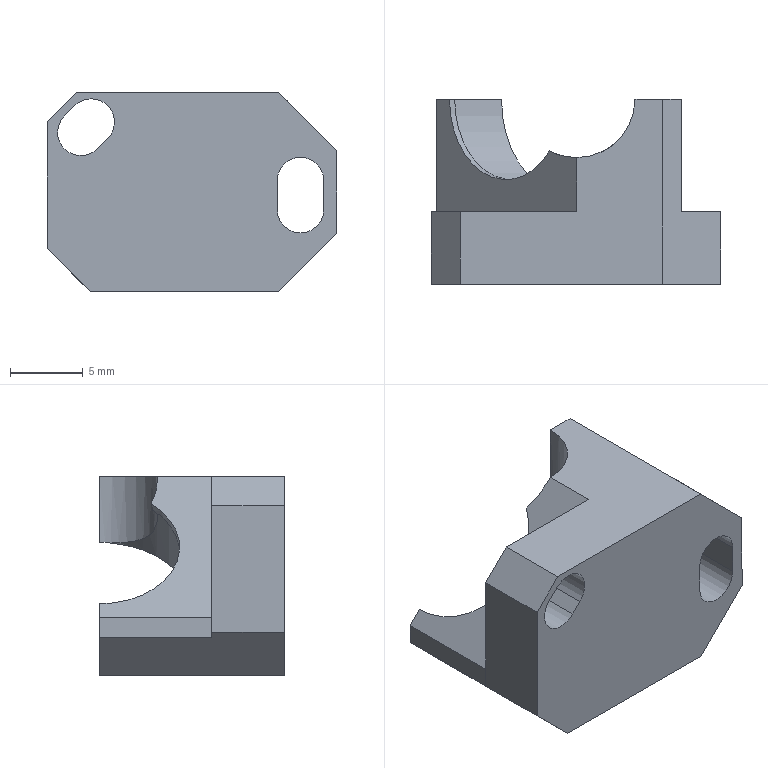Part | SolidWorks | features ICE 10, Chamfer 3, Extrusion 1, MoveFace 1 | 1 solid | 30 faces | box 19.9 x 12.7 x 13.659 mm | volume 1490 mm3 | plane 21 | cylinder 9 | commonest cylinder face diameters 3.2 x6 8 x1 11 x1 12.9 x1
STEP:
#1=CARTESIAN_POINT('',(8.727,0.,19.173));
#2=VERTEX_POINT('',#1);
#3=CARTESIAN_POINT('',(9.858,0.,16.442));
#4=VERTEX_POINT('',#3);
#5=CARTESIAN_POINT('',(8.727,0.,17.573));
#6=DIRECTION('',(0.,1.,0.));
#7=DIRECTION('',(0.,0.,1.));
#8=AXIS2_PLACEMENT_3D('',#5,#6,#7);
#9=CIRCLE('',#8,1.6);
#10=EDGE_CURVE('',#2,#4,#9,.T.);
#11=ORIENTED_EDGE('',*,*,#10,.F.);
#12=CARTESIAN_POINT('',(8.727,5.,19.173));
#13=VERTEX_POINT('',#12);
#14=CARTESIAN_POINT('',(8.727,-5.,19.173));
#15=DIRECTION('',(0.,1.,0.));
#16=VECTOR('',#15,1000.);
#17=LINE('',#14,#16);
#18=EDGE_CURVE('',#2,#13,#17,.T.);
#19=ORIENTED_EDGE('',*,*,#18,.T.);
#20=CARTESIAN_POINT('',(9.858,5.,16.442));
#21=VERTEX_POINT('',#20);
#22=CARTESIAN_POINT('',(8.727,5.,17.573));
#23=DIRECTION('',(0.,1.,0.));
#24=DIRECTION('',(0.,0.,1.));
#25=AXIS2_PLACEMENT_3D('',#22,#23,#24);
#26=CIRCLE('',#25,1.6);
#27=EDGE_CURVE('',#13,#21,#26,.T.);
#28=ORIENTED_EDGE('',*,*,#27,.T.);
#29=CARTESIAN_POINT('',(9.858,-5.,16.442));
#30=DIRECTION('',(0.,1.,0.));
#31=VECTOR('',#30,1000.);
#32=LINE('',#29,#31);
#33=EDGE_CURVE('',#4,#21,#32,.T.);
#34=ORIENTED_EDGE('',*,*,#33,.F.);
#35=EDGE_LOOP('',(#11,#19,#28,#34));
#36=FACE_OUTER_BOUND('',#35,.T.);
#37=CARTESIAN_POINT('',(8.727,-5.,17.573));
#38=DIRECTION('',(0.,1.,0.));
#39=DIRECTION('',(0.,0.,1.));
#40=AXIS2_PLACEMENT_3D('',#37,#38,#39);
#41=CYLINDRICAL_SURFACE('',#40,1.6);
#42=ADVANCED_FACE('',(#36),#41,.F.);
#43=CARTESIAN_POINT('',(23.1,0.,15.154));
#44=VERTEX_POINT('',#43);
#45=CARTESIAN_POINT('',(24.7,0.,13.554));
#46=VERTEX_POINT('',#45);
#47=CARTESIAN_POINT('',(23.1,0.,13.554));
#48=DIRECTION('',(0.,1.,0.));
#49=DIRECTION('',(0.,0.,1.));
#50=AXIS2_PLACEMENT_3D('',#47,#48,#49);
#51=CIRCLE('',#50,1.6);
#52=EDGE_CURVE('',#44,#46,#51,.T.);
#53=ORIENTED_EDGE('',*,*,#52,.F.);
#54=CARTESIAN_POINT('',(23.1,5.,15.154));
#55=VERTEX_POINT('',#54);
#56=CARTESIAN_POINT('',(23.1,-0.5,15.154));
#57=DIRECTION('',(0.,1.,0.));
#58=VECTOR('',#57,1000.);
#59=LINE('',#56,#58);
#60=EDGE_CURVE('',#44,#55,#59,.T.);
#61=ORIENTED_EDGE('',*,*,#60,.T.);
#62=CARTESIAN_POINT('',(24.7,5.,13.554));
#63=VERTEX_POINT('',#62);
#64=CARTESIAN_POINT('',(23.1,5.,13.554));
#65=DIRECTION('',(0.,1.,0.));
#66=DIRECTION('',(0.,0.,1.));
#67=AXIS2_PLACEMENT_3D('',#64,#65,#66);
#68=CIRCLE('',#67,1.6);
#69=EDGE_CURVE('',#55,#63,#68,.T.);
#70=ORIENTED_EDGE('',*,*,#69,.T.);
#71=CARTESIAN_POINT('',(24.7,-0.5,13.554));
#72=DIRECTION('',(0.,1.,0.));
#73=VECTOR('',#72,1000.);
#74=LINE('',#71,#73);
#75=EDGE_CURVE('',#46,#63,#74,.T.);
#76=ORIENTED_EDGE('',*,*,#75,.F.);
#77=EDGE_LOOP('',(#53,#61,#70,#76));
#78=FACE_OUTER_BOUND('',#77,.T.);
#79=CARTESIAN_POINT('',(23.1,-0.5,13.554));
#80=DIRECTION('',(0.,1.,0.));
#81=DIRECTION('',(0.,0.,1.));
#82=AXIS2_PLACEMENT_3D('',#79,#80,#81);
#83=CYLINDRICAL_SURFACE('',#82,1.6);
#84=ADVANCED_FACE('',(#78),#83,.F.);
#85=CARTESIAN_POINT('',(13.83,9.163,17.727));
#86=VERTEX_POINT('',#85);
#87=CARTESIAN_POINT('',(6.963,12.7,10.859));
#88=VERTEX_POINT('',#87);
#89=CARTESIAN_POINT('',(10.852,12.7,14.748));
#90=DIRECTION('',(0.7071,0.,-0.7071));
#91=DIRECTION('',(-0.7071,0.,-0.7071));
#92=AXIS2_PLACEMENT_3D('',#89,#90,#91);
#93=CIRCLE('',#92,5.5);
#94=EDGE_CURVE('',#86,#88,#93,.T.);
#95=ORIENTED_EDGE('',*,*,#94,.F.);
#96=CARTESIAN_POINT('',(14.106,9.031,17.288));
#97=VERTEX_POINT('',#96);
#98=CARTESIAN_POINT('',(13.83,9.163,17.727));
#99=CARTESIAN_POINT('',(13.92,9.116,17.58));
#100=CARTESIAN_POINT('',(14.012,9.072,17.434));
#101=CARTESIAN_POINT('',(14.106,9.031,17.288));
#102=B_SPLINE_CURVE_WITH_KNOTS('',3,(#98,#99,#100,#101),.UNSPECIFIED.,.F.,.F.,(4,4),(0.0005321,0.001067),.UNSPECIFIED.);
#103=EDGE_CURVE('',#86,#97,#102,.T.);
#104=ORIENTED_EDGE('',*,*,#103,.T.);
#105=CARTESIAN_POINT('',(7.32,12.7,10.502));
#106=VERTEX_POINT('',#105);
#107=CARTESIAN_POINT('',(11.209,12.7,14.391));
#108=DIRECTION('',(-0.7071,0.,0.7071));
#109=DIRECTION('',(-0.7071,0.,-0.7071));
#110=AXIS2_PLACEMENT_3D('',#107,#108,#109);
#111=CIRCLE('',#110,5.5);
#112=EDGE_CURVE('',#106,#97,#111,.T.);
#113=ORIENTED_EDGE('',*,*,#112,.F.);
#114=CARTESIAN_POINT('',(5.764,12.7,12.058));
#115=DIRECTION('',(-0.7071,0.,0.7071));
#116=VECTOR('',#115,1000.);
#117=LINE('',#114,#116);
#118=EDGE_CURVE('',#106,#88,#117,.T.);
#119=ORIENTED_EDGE('',*,*,#118,.T.);
#120=EDGE_LOOP('',(#95,#104,#113,#119));
#121=FACE_OUTER_BOUND('',#120,.T.);
#122=CARTESIAN_POINT('',(9.653,12.7,15.947));
#123=DIRECTION('',(0.7071,0.,-0.7071));
#124=DIRECTION('',(-0.7071,0.,-0.7071));
#125=AXIS2_PLACEMENT_3D('',#122,#123,#124);
#126=CYLINDRICAL_SURFACE('',#125,5.5);
#127=ADVANCED_FACE('',(#121),#126,.F.);
#128=CARTESIAN_POINT('',(19.699,12.7,19.6));
#129=VERTEX_POINT('',#128);
#130=CARTESIAN_POINT('',(19.699,12.7,15.103));
#131=VERTEX_POINT('',#130);
#132=CARTESIAN_POINT('',(19.699,12.7,5.6));
#133=DIRECTION('',(0.,0.,-1.));
#134=VECTOR('',#133,1000.);
#135=LINE('',#132,#134);
#136=EDGE_CURVE('',#129,#131,#135,.T.);
#137=ORIENTED_EDGE('',*,*,#136,.F.);
#138=CARTESIAN_POINT('',(21.6,12.7,19.6));
#139=VERTEX_POINT('',#138);
#140=CARTESIAN_POINT('',(0.,12.7,19.6));
#141=DIRECTION('',(-1.,0.,0.));
#142=VECTOR('',#141,1000.);
#143=LINE('',#140,#142);
#144=EDGE_CURVE('',#139,#129,#143,.T.);
#145=ORIENTED_EDGE('',*,*,#144,.F.);
#146=CARTESIAN_POINT('',(22.898,12.7,18.302));
#147=VERTEX_POINT('',#146);
#148=CARTESIAN_POINT('',(21.6,12.7,19.6));
#149=DIRECTION('',(-0.7071,0.,0.7071));
#150=VECTOR('',#149,1000.);
#151=LINE('',#148,#150);
#152=EDGE_CURVE('',#147,#139,#151,.T.);
#153=ORIENTED_EDGE('',*,*,#152,.F.);
#154=CARTESIAN_POINT('',(25.6,12.7,21.004));
#155=DIRECTION('',(-0.7071,0.,-0.7071));
#156=VECTOR('',#155,1000.);
#157=LINE('',#154,#156);
#158=EDGE_CURVE('',#147,#131,#157,.T.);
#159=ORIENTED_EDGE('',*,*,#158,.T.);
#160=EDGE_LOOP('',(#137,#145,#153,#159));
#161=FACE_OUTER_BOUND('',#160,.T.);
#162=CARTESIAN_POINT('',(0.,12.7,0.));
#163=DIRECTION('',(0.,1.,0.));
#164=DIRECTION('',(0.,0.,1.));
#165=AXIS2_PLACEMENT_3D('',#162,#163,#164);
#166=PLANE('',#165);
#167=ADVANCED_FACE('',(#161),#166,.T.);
#168=CARTESIAN_POINT('',(25.6,5.,15.6));
#169=VERTEX_POINT('',#168);
#170=CARTESIAN_POINT('',(22.898,5.,18.302));
#171=VERTEX_POINT('',#170);
#172=CARTESIAN_POINT('',(20.6,5.,20.6));
#173=DIRECTION('',(-0.7071,0.,0.7071));
#174=VECTOR('',#173,1000.);
#175=LINE('',#172,#174);
#176=EDGE_CURVE('',#169,#171,#175,.T.);
#177=ORIENTED_EDGE('',*,*,#176,.F.);
#178=CARTESIAN_POINT('',(25.6,5.,9.941));
#179=VERTEX_POINT('',#178);
#180=CARTESIAN_POINT('',(25.6,5.,0.));
#181=DIRECTION('',(0.,0.,-1.));
#182=VECTOR('',#181,1000.);
#183=LINE('',#180,#182);
#184=EDGE_CURVE('',#169,#179,#183,.T.);
#185=ORIENTED_EDGE('',*,*,#184,.T.);
#186=CARTESIAN_POINT('',(21.6,5.,5.941));
#187=VERTEX_POINT('',#186);
#188=CARTESIAN_POINT('',(7.829,5.,-7.829));
#189=DIRECTION('',(-0.7071,0.,-0.7071));
#190=VECTOR('',#189,1000.);
#191=LINE('',#188,#190);
#192=EDGE_CURVE('',#179,#187,#191,.T.);
#193=ORIENTED_EDGE('',*,*,#192,.T.);
#194=CARTESIAN_POINT('',(10.537,5.,5.941));
#195=VERTEX_POINT('',#194);
#196=CARTESIAN_POINT('',(0.,5.,5.941));
#197=DIRECTION('',(1.,0.,0.));
#198=VECTOR('',#197,1000.);
#199=LINE('',#196,#198);
#200=EDGE_CURVE('',#195,#187,#199,.T.);
#201=ORIENTED_EDGE('',*,*,#200,.F.);
#202=CARTESIAN_POINT('',(15.098,5.,10.502));
#203=DIRECTION('',(-0.7071,0.,-0.7071));
#204=VECTOR('',#203,1000.);
#205=LINE('',#202,#204);
#206=EDGE_CURVE('',#171,#195,#205,.T.);
#207=ORIENTED_EDGE('',*,*,#206,.F.);
#208=EDGE_LOOP('',(#177,#185,#193,#201,#207));
#209=FACE_OUTER_BOUND('',#208,.T.);
#210=CARTESIAN_POINT('',(21.5,5.,13.554));
#211=VERTEX_POINT('',#210);
#212=CARTESIAN_POINT('',(23.1,5.,13.554));
#213=DIRECTION('',(0.,1.,0.));
#214=DIRECTION('',(0.,0.,1.));
#215=AXIS2_PLACEMENT_3D('',#212,#213,#214);
#216=CIRCLE('',#215,1.6);
#217=EDGE_CURVE('',#211,#55,#216,.T.);
#218=ORIENTED_EDGE('',*,*,#217,.F.);
#219=CARTESIAN_POINT('',(21.5,5.,11.554));
#220=VERTEX_POINT('',#219);
#221=CARTESIAN_POINT('',(21.5,5.,13.554));
#222=DIRECTION('',(0.,0.,1.));
#223=VECTOR('',#222,1000.);
#224=LINE('',#221,#223);
#225=EDGE_CURVE('',#220,#211,#224,.T.);
#226=ORIENTED_EDGE('',*,*,#225,.F.);
#227=CARTESIAN_POINT('',(24.7,5.,11.554));
#228=VERTEX_POINT('',#227);
#229=CARTESIAN_POINT('',(23.1,5.,11.554));
#230=DIRECTION('',(0.,1.,0.));
#231=DIRECTION('',(0.,0.,1.));
#232=AXIS2_PLACEMENT_3D('',#229,#230,#231);
#233=CIRCLE('',#232,1.6);
#234=EDGE_CURVE('',#228,#220,#233,.T.);
#235=ORIENTED_EDGE('',*,*,#234,.F.);
#236=CARTESIAN_POINT('',(24.7,5.,13.554));
#237=DIRECTION('',(0.,0.,-1.));
#238=VECTOR('',#237,1000.);
#239=LINE('',#236,#238);
#240=EDGE_CURVE('',#63,#228,#239,.T.);
#241=ORIENTED_EDGE('',*,*,#240,.F.);
#242=ORIENTED_EDGE('',*,*,#69,.F.);
#243=EDGE_LOOP('',(#218,#226,#235,#241,#242));
#244=FACE_BOUND('',#243,.T.);
#245=CARTESIAN_POINT('',(0.,5.,0.));
#246=DIRECTION('',(0.,1.,0.));
#247=DIRECTION('',(0.,0.,1.));
#248=AXIS2_PLACEMENT_3D('',#245,#246,#247);
#249=PLANE('',#248);
#250=ADVANCED_FACE('',(#209,#244),#249,.T.);
#251=CARTESIAN_POINT('',(5.7,5.,17.6));
#252=VERTEX_POINT('',#251);
#253=CARTESIAN_POINT('',(5.7,5.,8.896));
#254=VERTEX_POINT('',#253);
#255=CARTESIAN_POINT('',(5.7,5.,0.));
#256=DIRECTION('',(0.,0.,-1.));
#257=VECTOR('',#256,1000.);
#258=LINE('',#255,#257);
#259=EDGE_CURVE('',#252,#254,#258,.T.);
#260=ORIENTED_EDGE('',*,*,#259,.F.);
#261=CARTESIAN_POINT('',(7.7,5.,19.6));
#262=VERTEX_POINT('',#261);
#263=CARTESIAN_POINT('',(-5.6,5.,6.3));
#264=DIRECTION('',(0.7071,0.,0.7071));
#265=VECTOR('',#264,1000.);
#266=LINE('',#263,#265);
#267=EDGE_CURVE('',#252,#262,#266,.T.);
#268=ORIENTED_EDGE('',*,*,#267,.T.);
#269=CARTESIAN_POINT('',(15.704,5.,19.6));
#270=VERTEX_POINT('',#269);
#271=CARTESIAN_POINT('',(0.,5.,19.6));
#272=DIRECTION('',(-1.,0.,0.));
#273=VECTOR('',#272,1000.);
#274=LINE('',#271,#273);
#275=EDGE_CURVE('',#270,#262,#274,.T.);
#276=ORIENTED_EDGE('',*,*,#275,.F.);
#277=CARTESIAN_POINT('',(6.054,5.,9.95));
#278=VERTEX_POINT('',#277);
#279=CARTESIAN_POINT('',(0.7,5.,4.596));
#280=DIRECTION('',(0.7071,0.,0.7071));
#281=VECTOR('',#280,1000.);
#282=LINE('',#279,#281);
#283=EDGE_CURVE('',#278,#270,#282,.T.);
#284=ORIENTED_EDGE('',*,*,#283,.F.);
#285=CARTESIAN_POINT('',(6.054,5.,8.543));
#286=VERTEX_POINT('',#285);
#287=CARTESIAN_POINT('',(6.054,5.,9.95));
#288=DIRECTION('',(0.,0.,-1.));
#289=VECTOR('',#288,1000.);
#290=LINE('',#287,#289);
#291=EDGE_CURVE('',#278,#286,#290,.T.);
#292=ORIENTED_EDGE('',*,*,#291,.T.);
#293=CARTESIAN_POINT('',(7.298,5.,7.298));
#294=DIRECTION('',(0.7071,0.,-0.7071));
#295=VECTOR('',#294,1000.);
#296=LINE('',#293,#295);
#297=EDGE_CURVE('',#254,#286,#296,.T.);
#298=ORIENTED_EDGE('',*,*,#297,.F.);
#299=EDGE_LOOP('',(#260,#268,#276,#284,#292,#298));
#300=FACE_OUTER_BOUND('',#299,.T.);
#301=CARTESIAN_POINT('',(7.596,5.,18.704));
#302=VERTEX_POINT('',#301);
#303=CARTESIAN_POINT('',(8.727,5.,17.573));
#304=DIRECTION('',(0.,1.,0.));
#305=DIRECTION('',(0.,0.,1.));
#306=AXIS2_PLACEMENT_3D('',#303,#304,#305);
#307=CIRCLE('',#306,1.6);
#308=EDGE_CURVE('',#302,#13,#307,.T.);
#309=ORIENTED_EDGE('',*,*,#308,.F.);
#310=CARTESIAN_POINT('',(6.889,5.,17.997));
#311=VERTEX_POINT('',#310);
#312=CARTESIAN_POINT('',(6.889,5.,17.997));
#313=DIRECTION('',(0.7071,0.,0.7071));
#314=VECTOR('',#313,1000.);
#315=LINE('',#312,#314);
#316=EDGE_CURVE('',#311,#302,#315,.T.);
#317=ORIENTED_EDGE('',*,*,#316,.F.);
#318=CARTESIAN_POINT('',(9.151,5.,15.734));
#319=VERTEX_POINT('',#318);
#320=CARTESIAN_POINT('',(8.02,5.,16.866));
#321=DIRECTION('',(0.,1.,0.));
#322=DIRECTION('',(0.,0.,1.));
#323=AXIS2_PLACEMENT_3D('',#320,#321,#322);
#324=CIRCLE('',#323,1.6);
#325=EDGE_CURVE('',#319,#311,#324,.T.);
#326=ORIENTED_EDGE('',*,*,#325,.F.);
#327=CARTESIAN_POINT('',(9.858,5.,16.442));
#328=DIRECTION('',(-0.7071,0.,-0.7071));
#329=VECTOR('',#328,1000.);
#330=LINE('',#327,#329);
#331=EDGE_CURVE('',#21,#319,#330,.T.);
#332=ORIENTED_EDGE('',*,*,#331,.F.);
#333=ORIENTED_EDGE('',*,*,#27,.F.);
#334=EDGE_LOOP('',(#309,#317,#326,#332,#333));
#335=FACE_BOUND('',#334,.T.);
#336=CARTESIAN_POINT('',(0.,5.,0.));
#337=DIRECTION('',(0.,1.,0.));
#338=DIRECTION('',(0.,0.,1.));
#339=AXIS2_PLACEMENT_3D('',#336,#337,#338);
#340=PLANE('',#339);
#341=ADVANCED_FACE('',(#300,#335),#340,.T.);
#342=ORIENTED_EDGE('',*,*,#184,.F.);
#343=CARTESIAN_POINT('',(25.6,0.,15.6));
#344=VERTEX_POINT('',#343);
#345=CARTESIAN_POINT('',(25.6,-17.8,15.6));
#346=DIRECTION('',(0.,1.,0.));
#347=VECTOR('',#346,1000.);
#348=LINE('',#345,#347);
#349=EDGE_CURVE('',#344,#169,#348,.T.);
#350=ORIENTED_EDGE('',*,*,#349,.F.);
#351=CARTESIAN_POINT('',(25.6,0.,9.941));
#352=VERTEX_POINT('',#351);
#353=CARTESIAN_POINT('',(25.6,0.,0.));
#354=DIRECTION('',(0.,0.,-1.));
#355=VECTOR('',#354,1000.);
#356=LINE('',#353,#355);
#357=EDGE_CURVE('',#344,#352,#356,.T.);
#358=ORIENTED_EDGE('',*,*,#357,.T.);
#359=CARTESIAN_POINT('',(25.6,5.,9.941));
#360=DIRECTION('',(0.,1.,0.));
#361=VECTOR('',#360,1000.);
#362=LINE('',#359,#361);
#363=EDGE_CURVE('',#352,#179,#362,.T.);
#364=ORIENTED_EDGE('',*,*,#363,.T.);
#365=EDGE_LOOP('',(#342,#350,#358,#364));
#366=FACE_OUTER_BOUND('',#365,.T.);
#367=CARTESIAN_POINT('',(25.6,5.,0.));
#368=DIRECTION('',(-1.,0.,0.));
#369=DIRECTION('',(0.,0.,1.));
#370=AXIS2_PLACEMENT_3D('',#367,#368,#369);
#371=PLANE('',#370);
#372=ADVANCED_FACE('',(#366),#371,.F.);
#373=CARTESIAN_POINT('',(6.889,0.,17.997));
#374=VERTEX_POINT('',#373);
#375=CARTESIAN_POINT('',(7.596,0.,18.704));
#376=VERTEX_POINT('',#375);
#377=CARTESIAN_POINT('',(-5.204,0.,5.904));
#378=DIRECTION('',(0.7071,0.,0.7071));
#379=VECTOR('',#378,1000.);
#380=LINE('',#377,#379);
#381=EDGE_CURVE('',#374,#376,#380,.T.);
#382=ORIENTED_EDGE('',*,*,#381,.T.);
#383=CARTESIAN_POINT('',(8.727,0.,17.573));
#384=DIRECTION('',(0.,1.,0.));
#385=DIRECTION('',(0.,0.,1.));
#386=AXIS2_PLACEMENT_3D('',#383,#384,#385);
#387=CIRCLE('',#386,1.6);
#388=EDGE_CURVE('',#376,#2,#387,.T.);
#389=ORIENTED_EDGE('',*,*,#388,.T.);
#390=ORIENTED_EDGE('',*,*,#10,.T.);
#391=CARTESIAN_POINT('',(9.151,0.,15.734));
#392=VERTEX_POINT('',#391);
#393=CARTESIAN_POINT('',(-2.942,0.,3.642));
#394=DIRECTION('',(-0.7071,0.,-0.7071));
#395=VECTOR('',#394,1000.);
#396=LINE('',#393,#395);
#397=EDGE_CURVE('',#4,#392,#396,.T.);
#398=ORIENTED_EDGE('',*,*,#397,.T.);
#399=CARTESIAN_POINT('',(8.02,0.,16.866));
#400=DIRECTION('',(0.,1.,0.));
#401=DIRECTION('',(0.,0.,1.));
#402=AXIS2_PLACEMENT_3D('',#399,#400,#401);
#403=CIRCLE('',#402,1.6);
#404=EDGE_CURVE('',#392,#374,#403,.T.);
#405=ORIENTED_EDGE('',*,*,#404,.T.);
#406=EDGE_LOOP('',(#382,#389,#390,#398,#405));
#407=FACE_BOUND('',#406,.T.);
#408=CARTESIAN_POINT('',(21.5,0.,11.554));
#409=VERTEX_POINT('',#408);
#410=CARTESIAN_POINT('',(21.5,0.,13.554));
#411=VERTEX_POINT('',#410);
#412=CARTESIAN_POINT('',(21.5,0.,0.));
#413=DIRECTION('',(0.,0.,1.));
#414=VECTOR('',#413,1000.);
#415=LINE('',#412,#414);
#416=EDGE_CURVE('',#409,#411,#415,.T.);
#417=ORIENTED_EDGE('',*,*,#416,.T.);
#418=CARTESIAN_POINT('',(23.1,0.,13.554));
#419=DIRECTION('',(0.,1.,0.));
#420=DIRECTION('',(0.,0.,1.));
#421=AXIS2_PLACEMENT_3D('',#418,#419,#420);
#422=CIRCLE('',#421,1.6);
#423=EDGE_CURVE('',#411,#44,#422,.T.);
#424=ORIENTED_EDGE('',*,*,#423,.T.);
#425=ORIENTED_EDGE('',*,*,#52,.T.);
#426=CARTESIAN_POINT('',(24.7,0.,11.554));
#427=VERTEX_POINT('',#426);
#428=CARTESIAN_POINT('',(24.7,0.,0.));
#429=DIRECTION('',(0.,0.,-1.));
#430=VECTOR('',#429,1000.);
#431=LINE('',#428,#430);
#432=EDGE_CURVE('',#46,#427,#431,.T.);
#433=ORIENTED_EDGE('',*,*,#432,.T.);
#434=CARTESIAN_POINT('',(23.1,0.,11.554));
#435=DIRECTION('',(0.,1.,0.));
#436=DIRECTION('',(0.,0.,1.));
#437=AXIS2_PLACEMENT_3D('',#434,#435,#436);
#438=CIRCLE('',#437,1.6);
#439=EDGE_CURVE('',#427,#409,#438,.T.);
#440=ORIENTED_EDGE('',*,*,#439,.T.);
#441=EDGE_LOOP('',(#417,#424,#425,#433,#440));
#442=FACE_BOUND('',#441,.T.);
#443=CARTESIAN_POINT('',(21.6,0.,19.6));
#444=VERTEX_POINT('',#443);
#445=CARTESIAN_POINT('',(7.7,0.,19.6));
#446=VERTEX_POINT('',#445);
#447=CARTESIAN_POINT('',(0.,0.,19.6));
#448=DIRECTION('',(-1.,0.,0.));
#449=VECTOR('',#448,1000.);
#450=LINE('',#447,#449);
#451=EDGE_CURVE('',#444,#446,#450,.T.);
#452=ORIENTED_EDGE('',*,*,#451,.T.);
#453=CARTESIAN_POINT('',(5.7,0.,17.6));
#454=VERTEX_POINT('',#453);
#455=CARTESIAN_POINT('',(7.7,0.,19.6));
#456=DIRECTION('',(-0.7071,0.,-0.7071));
#457=VECTOR('',#456,1000.);
#458=LINE('',#455,#457);
#459=EDGE_CURVE('',#446,#454,#458,.T.);
#460=ORIENTED_EDGE('',*,*,#459,.T.);
#461=CARTESIAN_POINT('',(5.7,0.,8.896));
#462=VERTEX_POINT('',#461);
#463=CARTESIAN_POINT('',(5.7,0.,0.));
#464=DIRECTION('',(0.,0.,-1.));
#465=VECTOR('',#464,1000.);
#466=LINE('',#463,#465);
#467=EDGE_CURVE('',#454,#462,#466,.T.);
#468=ORIENTED_EDGE('',*,*,#467,.T.);
#469=CARTESIAN_POINT('',(8.655,0.,5.941));
#470=VERTEX_POINT('',#469);
#471=CARTESIAN_POINT('',(7.298,0.,7.298));
#472=DIRECTION('',(0.7071,0.,-0.7071));
#473=VECTOR('',#472,1000.);
#474=LINE('',#471,#473);
#475=EDGE_CURVE('',#462,#470,#474,.T.);
#476=ORIENTED_EDGE('',*,*,#475,.T.);
#477=CARTESIAN_POINT('',(21.6,0.,5.941));
#478=VERTEX_POINT('',#477);
#479=CARTESIAN_POINT('',(0.,0.,5.941));
#480=DIRECTION('',(1.,0.,0.));
#481=VECTOR('',#480,1000.);
#482=LINE('',#479,#481);
#483=EDGE_CURVE('',#470,#478,#482,.T.);
#484=ORIENTED_EDGE('',*,*,#483,.T.);
#485=CARTESIAN_POINT('',(25.6,0.,9.941));
#486=DIRECTION('',(0.7071,0.,0.7071));
#487=VECTOR('',#486,1000.);
#488=LINE('',#485,#487);
#489=EDGE_CURVE('',#478,#352,#488,.T.);
#490=ORIENTED_EDGE('',*,*,#489,.T.);
#491=ORIENTED_EDGE('',*,*,#357,.F.);
#492=CARTESIAN_POINT('',(20.6,0.,20.6));
#493=DIRECTION('',(-0.7071,0.,0.7071));
#494=VECTOR('',#493,1000.);
#495=LINE('',#492,#494);
#496=EDGE_CURVE('',#344,#444,#495,.T.);
#497=ORIENTED_EDGE('',*,*,#496,.T.);
#498=EDGE_LOOP('',(#452,#460,#468,#476,#484,#490,#491,#497));
#499=FACE_OUTER_BOUND('',#498,.T.);
#500=CARTESIAN_POINT('',(0.,0.,0.));
#501=DIRECTION('',(0.,1.,0.));
#502=DIRECTION('',(0.,0.,1.));
#503=AXIS2_PLACEMENT_3D('',#500,#501,#502);
#504=PLANE('',#503);
#505=ADVANCED_FACE('',(#407,#442,#499),#504,.F.);
#506=CARTESIAN_POINT('',(19.628,11.948,15.032));
#507=VERTEX_POINT('',#506);
#508=CARTESIAN_POINT('',(10.537,12.7,5.941));
#509=VERTEX_POINT('',#508);
#510=CARTESIAN_POINT('',(15.098,12.7,10.502));
#511=DIRECTION('',(0.7071,0.,-0.7071));
#512=DIRECTION('',(-0.7071,0.,-0.7071));
#513=AXIS2_PLACEMENT_3D('',#510,#511,#512);
#514=CIRCLE('',#513,6.45);
#515=EDGE_CURVE('',#507,#509,#514,.T.);
#516=ORIENTED_EDGE('',*,*,#515,.F.);
#517=CARTESIAN_POINT('',(19.628,11.948,15.032));
#518=CARTESIAN_POINT('',(19.675,12.196,15.079));
#519=CARTESIAN_POINT('',(19.699,12.448,15.103));
#520=CARTESIAN_POINT('',(19.699,12.7,15.103));
#521=(BOUNDED_CURVE()B_SPLINE_CURVE(3,(#517,#518,#519,#520),.UNSPECIFIED.,.F.,.F.)B_SPLINE_CURVE_WITH_KNOTS((4,4),(6.094,6.283),.UNSPECIFIED.)CURVE()GEOMETRIC_REPRESENTATION_ITEM()RATIONAL_B_SPLINE_CURVE((1.,0.997,0.997,1.))REPRESENTATION_ITEM(''));
#522=EDGE_CURVE('',#507,#131,#521,.T.);
#523=ORIENTED_EDGE('',*,*,#522,.T.);
#524=ORIENTED_EDGE('',*,*,#158,.F.);
#525=CARTESIAN_POINT('',(22.898,12.7,18.302));
#526=DIRECTION('',(0.,-1.,0.));
#527=VECTOR('',#526,1000.);
#528=LINE('',#525,#527);
#529=EDGE_CURVE('',#147,#171,#528,.T.);
#530=ORIENTED_EDGE('',*,*,#529,.T.);
#531=ORIENTED_EDGE('',*,*,#206,.T.);
#532=CARTESIAN_POINT('',(10.537,12.7,5.941));
#533=DIRECTION('',(0.,1.,0.));
#534=VECTOR('',#533,1000.);
#535=LINE('',#532,#534);
#536=EDGE_CURVE('',#195,#509,#535,.T.);
#537=ORIENTED_EDGE('',*,*,#536,.T.);
#538=EDGE_LOOP('',(#516,#523,#524,#530,#531,#537));
#539=FACE_OUTER_BOUND('',#538,.T.);
#540=CARTESIAN_POINT('',(15.098,12.7,10.502));
#541=DIRECTION('',(-0.7071,0.,0.7071));
#542=DIRECTION('',(0.7071,0.,0.7071));
#543=AXIS2_PLACEMENT_3D('',#540,#541,#542);
#544=PLANE('',#543);
#545=ADVANCED_FACE('',(#539),#544,.F.);
#546=CARTESIAN_POINT('',(6.054,12.7,9.95));
#547=VERTEX_POINT('',#546);
#548=CARTESIAN_POINT('',(0.7,12.7,4.596));
#549=DIRECTION('',(0.7071,0.,0.7071));
#550=VECTOR('',#549,1000.);
#551=LINE('',#548,#550);
#552=EDGE_CURVE('',#547,#88,#551,.T.);
#553=ORIENTED_EDGE('',*,*,#552,.F.);
#554=CARTESIAN_POINT('',(6.054,12.7,9.95));
#555=DIRECTION('',(0.,-1.,0.));
#556=VECTOR('',#555,1000.);
#557=LINE('',#554,#556);
#558=EDGE_CURVE('',#547,#278,#557,.T.);
#559=ORIENTED_EDGE('',*,*,#558,.T.);
#560=ORIENTED_EDGE('',*,*,#283,.T.);
#561=CARTESIAN_POINT('',(15.704,8.7,19.6));
#562=VERTEX_POINT('',#561);
#563=CARTESIAN_POINT('',(15.704,12.7,19.6));
#564=DIRECTION('',(0.,1.,0.));
#565=VECTOR('',#564,1000.);
#566=LINE('',#563,#565);
#567=EDGE_CURVE('',#270,#562,#566,.T.);
#568=ORIENTED_EDGE('',*,*,#567,.T.);
#569=CARTESIAN_POINT('',(15.704,8.7,19.6));
#570=CARTESIAN_POINT('',(15.048,8.699,18.944));
#571=CARTESIAN_POINT('',(14.411,8.857,18.307));
#572=CARTESIAN_POINT('',(13.83,9.163,17.727));
#573=(BOUNDED_CURVE()B_SPLINE_CURVE(3,(#569,#570,#571,#572),.UNSPECIFIED.,.F.,.T.)B_SPLINE_CURVE_WITH_KNOTS((4,4),(1.57,2.057),.UNSPECIFIED.)CURVE()GEOMETRIC_REPRESENTATION_ITEM()RATIONAL_B_SPLINE_CURVE((1.,0.9803,0.9803,1.))REPRESENTATION_ITEM(''));
#574=EDGE_CURVE('',#562,#86,#573,.T.);
#575=ORIENTED_EDGE('',*,*,#574,.T.);
#576=ORIENTED_EDGE('',*,*,#94,.T.);
#577=EDGE_LOOP('',(#553,#559,#560,#568,#575,#576));
#578=FACE_OUTER_BOUND('',#577,.T.);
#579=CARTESIAN_POINT('',(0.7,12.7,4.596));
#580=DIRECTION('',(0.7071,0.,-0.7071));
#581=DIRECTION('',(-0.7071,0.,-0.7071));
#582=AXIS2_PLACEMENT_3D('',#579,#580,#581);
#583=PLANE('',#582);
#584=ADVANCED_FACE('',(#578),#583,.F.);
#585=CARTESIAN_POINT('',(6.054,12.7,8.543));
#586=VERTEX_POINT('',#585);
#587=CARTESIAN_POINT('',(8.655,12.7,5.941));
#588=VERTEX_POINT('',#587);
#589=CARTESIAN_POINT('',(5.,12.7,9.596));
#590=DIRECTION('',(0.7071,0.,-0.7071));
#591=VECTOR('',#590,1000.);
#592=LINE('',#589,#591);
#593=EDGE_CURVE('',#586,#588,#592,.T.);
#594=ORIENTED_EDGE('',*,*,#593,.F.);
#595=CARTESIAN_POINT('',(6.054,12.7,0.));
#596=DIRECTION('',(0.,0.,1.));
#597=VECTOR('',#596,1000.);
#598=LINE('',#595,#597);
#599=EDGE_CURVE('',#586,#547,#598,.T.);
#600=ORIENTED_EDGE('',*,*,#599,.T.);
#601=ORIENTED_EDGE('',*,*,#552,.T.);
#602=ORIENTED_EDGE('',*,*,#118,.F.);
#603=CARTESIAN_POINT('',(6.648,12.7,9.83));
#604=VERTEX_POINT('',#603);
#605=CARTESIAN_POINT('',(-1.591,12.7,1.591));
#606=DIRECTION('',(-0.7071,0.,-0.7071));
#607=VECTOR('',#606,1000.);
#608=LINE('',#605,#607);
#609=EDGE_CURVE('',#106,#604,#608,.T.);
#610=ORIENTED_EDGE('',*,*,#609,.T.);
#611=CARTESIAN_POINT('',(6.648,12.7,9.83));
#612=DIRECTION('',(-0.7071,0.,0.7071));
#613=VECTOR('',#612,1000.);
#614=LINE('',#611,#613);
#615=EDGE_CURVE('',#509,#604,#614,.T.);
#616=ORIENTED_EDGE('',*,*,#615,.F.);
#617=CARTESIAN_POINT('',(10.537,12.7,5.941));
#618=DIRECTION('',(1.,0.,0.));
#619=VECTOR('',#618,1000.);
#620=LINE('',#617,#619);
#621=EDGE_CURVE('',#588,#509,#620,.T.);
#622=ORIENTED_EDGE('',*,*,#621,.F.);
#623=EDGE_LOOP('',(#594,#600,#601,#602,#610,#616,#622));
#624=FACE_OUTER_BOUND('',#623,.T.);
#625=CARTESIAN_POINT('',(0.,12.7,0.));
#626=DIRECTION('',(0.,1.,0.));
#627=DIRECTION('',(0.,0.,1.));
#628=AXIS2_PLACEMENT_3D('',#625,#626,#627);
#629=PLANE('',#628);
#630=ADVANCED_FACE('',(#624),#629,.T.);
#631=CARTESIAN_POINT('',(14.838,8.794,18.02));
#632=VERTEX_POINT('',#631);
#633=CARTESIAN_POINT('',(11.209,12.7,14.391));
#634=DIRECTION('',(0.7071,0.,-0.7071));
#635=DIRECTION('',(-0.7071,0.,-0.7071));
#636=AXIS2_PLACEMENT_3D('',#633,#634,#635);
#637=CIRCLE('',#636,6.45);
#638=EDGE_CURVE('',#632,#604,#637,.T.);
#639=ORIENTED_EDGE('',*,*,#638,.F.);
#640=CARTESIAN_POINT('',(14.838,8.794,18.02));
#641=CARTESIAN_POINT('',(15.222,8.709,17.546));
#642=CARTESIAN_POINT('',(15.632,8.674,17.095));
#643=CARTESIAN_POINT('',(16.32,8.742,16.483));
#644=CARTESIAN_POINT('',(16.559,8.785,16.291));
#645=CARTESIAN_POINT('',(16.925,8.891,16.036));
#646=CARTESIAN_POINT('',(17.049,8.932,15.955));
#647=CARTESIAN_POINT('',(17.299,9.031,15.804));
#648=CARTESIAN_POINT('',(17.425,9.089,15.734));
#649=CARTESIAN_POINT('',(17.796,9.282,15.543));
#650=CARTESIAN_POINT('',(18.036,9.44,15.441));
#651=CARTESIAN_POINT('',(18.378,9.726,15.317));
#652=CARTESIAN_POINT('',(18.489,9.829,15.282));
#653=CARTESIAN_POINT('',(18.696,10.047,15.22));
#654=CARTESIAN_POINT('',(18.794,10.161,15.193));
#655=CARTESIAN_POINT('',(19.069,10.524,15.126));
#656=CARTESIAN_POINT('',(19.228,10.791,15.095));
#657=CARTESIAN_POINT('',(19.477,11.349,15.052));
#658=CARTESIAN_POINT('',(19.57,11.644,15.039));
#659=CARTESIAN_POINT('',(19.628,11.948,15.032));
#660=B_SPLINE_CURVE_WITH_KNOTS('',3,(#640,#641,#642,#643,#644,#645,#646,#647,#648,#649,#650,#651,#652,#653,#654,#655,#656,#657,#658,#659),.UNSPECIFIED.,.F.,.F.,(4,2,2,2,2,2,2,2,2,4),(0.,0.001831,0.002746,0.003203,0.003661,0.004576,0.005034,0.005492,0.006407,0.007322),.UNSPECIFIED.);
#661=EDGE_CURVE('',#632,#507,#660,.T.);
#662=ORIENTED_EDGE('',*,*,#661,.T.);
#663=ORIENTED_EDGE('',*,*,#515,.T.);
#664=ORIENTED_EDGE('',*,*,#615,.T.);
#665=EDGE_LOOP('',(#639,#662,#663,#664));
#666=FACE_OUTER_BOUND('',#665,.T.);
#667=CARTESIAN_POINT('',(11.209,12.7,14.391));
#668=DIRECTION('',(0.7071,0.,-0.7071));
#669=DIRECTION('',(-0.7071,0.,-0.7071));
#670=AXIS2_PLACEMENT_3D('',#667,#668,#669);
#671=CYLINDRICAL_SURFACE('',#670,6.45);
#672=ADVANCED_FACE('',(#666),#671,.F.);
#673=CARTESIAN_POINT('',(14.838,8.794,18.02));
#674=CARTESIAN_POINT('',(14.587,8.849,17.769));
#675=CARTESIAN_POINT('',(14.342,8.928,17.524));
#676=CARTESIAN_POINT('',(14.106,9.031,17.288));
#677=(BOUNDED_CURVE()B_SPLINE_CURVE(3,(#673,#674,#675,#676),.UNSPECIFIED.,.F.,.T.)B_SPLINE_CURVE_WITH_KNOTS((4,4),(1.788,1.98),.UNSPECIFIED.)CURVE()GEOMETRIC_REPRESENTATION_ITEM()RATIONAL_B_SPLINE_CURVE((1.,0.9969,0.9969,1.))REPRESENTATION_ITEM(''));
#678=EDGE_CURVE('',#632,#97,#677,.T.);
#679=ORIENTED_EDGE('',*,*,#678,.F.);
#680=ORIENTED_EDGE('',*,*,#638,.T.);
#681=ORIENTED_EDGE('',*,*,#609,.F.);
#682=ORIENTED_EDGE('',*,*,#112,.T.);
#683=EDGE_LOOP('',(#679,#680,#681,#682));
#684=FACE_OUTER_BOUND('',#683,.T.);
#685=CARTESIAN_POINT('',(11.209,12.7,14.391));
#686=DIRECTION('',(0.7071,0.,-0.7071));
#687=DIRECTION('',(-0.7071,0.,-0.7071));
#688=AXIS2_PLACEMENT_3D('',#685,#686,#687);
#689=PLANE('',#688);
#690=ADVANCED_FACE('',(#684),#689,.T.);
#691=ORIENTED_EDGE('',*,*,#60,.F.);
#692=ORIENTED_EDGE('',*,*,#423,.F.);
#693=CARTESIAN_POINT('',(21.5,-0.5,13.554));
#694=DIRECTION('',(0.,1.,0.));
#695=VECTOR('',#694,1000.);
#696=LINE('',#693,#695);
#697=EDGE_CURVE('',#411,#211,#696,.T.);
#698=ORIENTED_EDGE('',*,*,#697,.T.);
#699=ORIENTED_EDGE('',*,*,#217,.T.);
#700=EDGE_LOOP('',(#691,#692,#698,#699));
#701=FACE_OUTER_BOUND('',#700,.T.);
#702=CARTESIAN_POINT('',(23.1,-0.5,13.554));
#703=DIRECTION('',(0.,1.,0.));
#704=DIRECTION('',(0.,0.,1.));
#705=AXIS2_PLACEMENT_3D('',#702,#703,#704);
#706=CYLINDRICAL_SURFACE('',#705,1.6);
#707=ADVANCED_FACE('',(#701),#706,.F.);
#708=CARTESIAN_POINT('',(21.5,-0.5,11.554));
#709=DIRECTION('',(0.,1.,0.));
#710=VECTOR('',#709,1000.);
#711=LINE('',#708,#710);
#712=EDGE_CURVE('',#409,#220,#711,.T.);
#713=ORIENTED_EDGE('',*,*,#712,.T.);
#714=ORIENTED_EDGE('',*,*,#225,.T.);
#715=ORIENTED_EDGE('',*,*,#697,.F.);
#716=ORIENTED_EDGE('',*,*,#416,.F.);
#717=EDGE_LOOP('',(#713,#714,#715,#716));
#718=FACE_OUTER_BOUND('',#717,.T.);
#719=CARTESIAN_POINT('',(21.5,-0.5,13.554));
#720=DIRECTION('',(-1.,0.,0.));
#721=DIRECTION('',(0.,0.,1.));
#722=AXIS2_PLACEMENT_3D('',#719,#720,#721);
#723=PLANE('',#722);
#724=ADVANCED_FACE('',(#718),#723,.F.);
#725=CARTESIAN_POINT('',(24.7,-0.5,11.554));
#726=DIRECTION('',(0.,1.,0.));
#727=VECTOR('',#726,1000.);
#728=LINE('',#725,#727);
#729=EDGE_CURVE('',#427,#228,#728,.T.);
#730=ORIENTED_EDGE('',*,*,#729,.T.);
#731=ORIENTED_EDGE('',*,*,#234,.T.);
#732=ORIENTED_EDGE('',*,*,#712,.F.);
#733=ORIENTED_EDGE('',*,*,#439,.F.);
#734=EDGE_LOOP('',(#730,#731,#732,#733));
#735=FACE_OUTER_BOUND('',#734,.T.);
#736=CARTESIAN_POINT('',(23.1,-0.5,11.554));
#737=DIRECTION('',(0.,1.,0.));
#738=DIRECTION('',(0.,0.,1.));
#739=AXIS2_PLACEMENT_3D('',#736,#737,#738);
#740=CYLINDRICAL_SURFACE('',#739,1.6);
#741=ADVANCED_FACE('',(#735),#740,.F.);
#742=ORIENTED_EDGE('',*,*,#75,.T.);
#743=ORIENTED_EDGE('',*,*,#240,.T.);
#744=ORIENTED_EDGE('',*,*,#729,.F.);
#745=ORIENTED_EDGE('',*,*,#432,.F.);
#746=EDGE_LOOP('',(#742,#743,#744,#745));
#747=FACE_OUTER_BOUND('',#746,.T.);
#748=CARTESIAN_POINT('',(24.7,-0.5,13.554));
#749=DIRECTION('',(1.,0.,0.));
#750=DIRECTION('',(0.,0.,-1.));
#751=AXIS2_PLACEMENT_3D('',#748,#749,#750);
#752=PLANE('',#751);
#753=ADVANCED_FACE('',(#747),#752,.F.);
#754=ORIENTED_EDGE('',*,*,#483,.F.);
#755=CARTESIAN_POINT('',(8.655,-2.8,5.941));
#756=DIRECTION('',(0.,1.,0.));
#757=VECTOR('',#756,1000.);
#758=LINE('',#755,#757);
#759=EDGE_CURVE('',#470,#588,#758,.T.);
#760=ORIENTED_EDGE('',*,*,#759,.T.);
#761=ORIENTED_EDGE('',*,*,#621,.T.);
#762=ORIENTED_EDGE('',*,*,#536,.F.);
#763=ORIENTED_EDGE('',*,*,#200,.T.);
#764=CARTESIAN_POINT('',(21.6,-17.8,5.941));
#765=DIRECTION('',(0.,-1.,0.));
#766=VECTOR('',#765,1000.);
#767=LINE('',#764,#766);
#768=EDGE_CURVE('',#187,#478,#767,.T.);
#769=ORIENTED_EDGE('',*,*,#768,.T.);
#770=EDGE_LOOP('',(#754,#760,#761,#762,#763,#769));
#771=FACE_OUTER_BOUND('',#770,.T.);
#772=CARTESIAN_POINT('',(10.537,-17.8,5.941));
#773=DIRECTION('',(0.,0.,1.));
#774=DIRECTION('',(1.,0.,0.));
#775=AXIS2_PLACEMENT_3D('',#772,#773,#774);
#776=PLANE('',#775);
#777=ADVANCED_FACE('',(#771),#776,.F.);
#778=ORIENTED_EDGE('',*,*,#275,.T.);
#779=CARTESIAN_POINT('',(7.7,-17.8,19.6));
#780=DIRECTION('',(0.,-1.,0.));
#781=VECTOR('',#780,1000.);
#782=LINE('',#779,#781);
#783=EDGE_CURVE('',#262,#446,#782,.T.);
#784=ORIENTED_EDGE('',*,*,#783,.T.);
#785=ORIENTED_EDGE('',*,*,#451,.F.);
#786=CARTESIAN_POINT('',(21.6,-17.8,19.6));
#787=DIRECTION('',(0.,1.,0.));
#788=VECTOR('',#787,1000.);
#789=LINE('',#786,#788);
#790=EDGE_CURVE('',#444,#139,#789,.T.);
#791=ORIENTED_EDGE('',*,*,#790,.T.);
#792=ORIENTED_EDGE('',*,*,#144,.T.);
#793=CARTESIAN_POINT('',(15.699,12.7,19.6));
#794=DIRECTION('',(0.,0.,-1.));
#795=DIRECTION('',(-1.,0.,0.));
#796=AXIS2_PLACEMENT_3D('',#793,#794,#795);
#797=CIRCLE('',#796,4.);
#798=EDGE_CURVE('',#129,#562,#797,.T.);
#799=ORIENTED_EDGE('',*,*,#798,.T.);
#800=ORIENTED_EDGE('',*,*,#567,.F.);
#801=EDGE_LOOP('',(#778,#784,#785,#791,#792,#799,#800));
#802=FACE_OUTER_BOUND('',#801,.T.);
#803=CARTESIAN_POINT('',(0.,-17.8,19.6));
#804=DIRECTION('',(0.,0.,-1.));
#805=DIRECTION('',(-1.,0.,0.));
#806=AXIS2_PLACEMENT_3D('',#803,#804,#805);
#807=PLANE('',#806);
#808=ADVANCED_FACE('',(#802),#807,.F.);
#809=ORIENTED_EDGE('',*,*,#489,.F.);
#810=ORIENTED_EDGE('',*,*,#768,.F.);
#811=ORIENTED_EDGE('',*,*,#192,.F.);
#812=ORIENTED_EDGE('',*,*,#363,.F.);
#813=EDGE_LOOP('',(#809,#810,#811,#812));
#814=FACE_OUTER_BOUND('',#813,.T.);
#815=CARTESIAN_POINT('',(25.6,5.,9.941));
#816=DIRECTION('',(-0.7071,0.,0.7071));
#817=DIRECTION('',(0.,1.,0.));
#818=AXIS2_PLACEMENT_3D('',#815,#816,#817);
#819=PLANE('',#818);
#820=ADVANCED_FACE('',(#814),#819,.F.);
#821=ORIENTED_EDGE('',*,*,#349,.T.);
#822=ORIENTED_EDGE('',*,*,#176,.T.);
#823=ORIENTED_EDGE('',*,*,#529,.F.);
#824=ORIENTED_EDGE('',*,*,#152,.T.);
#825=ORIENTED_EDGE('',*,*,#790,.F.);
#826=ORIENTED_EDGE('',*,*,#496,.F.);
#827=EDGE_LOOP('',(#821,#822,#823,#824,#825,#826));
#828=FACE_OUTER_BOUND('',#827,.T.);
#829=CARTESIAN_POINT('',(21.6,-17.8,19.6));
#830=DIRECTION('',(-0.7071,0.,-0.7071));
#831=DIRECTION('',(-0.7071,0.,0.7071));
#832=AXIS2_PLACEMENT_3D('',#829,#830,#831);
#833=PLANE('',#832);
#834=ADVANCED_FACE('',(#828),#833,.F.);
#835=ORIENTED_EDGE('',*,*,#798,.F.);
#836=ORIENTED_EDGE('',*,*,#136,.T.);
#837=ORIENTED_EDGE('',*,*,#522,.F.);
#838=ORIENTED_EDGE('',*,*,#661,.F.);
#839=ORIENTED_EDGE('',*,*,#678,.T.);
#840=ORIENTED_EDGE('',*,*,#103,.F.);
#841=ORIENTED_EDGE('',*,*,#574,.F.);
#842=EDGE_LOOP('',(#835,#836,#837,#838,#839,#840,#841));
#843=FACE_OUTER_BOUND('',#842,.T.);
#844=CARTESIAN_POINT('',(15.699,12.7,5.6));
#845=DIRECTION('',(0.,0.,1.));
#846=DIRECTION('',(1.,0.,0.));
#847=AXIS2_PLACEMENT_3D('',#844,#845,#846);
#848=CYLINDRICAL_SURFACE('',#847,4.);
#849=ADVANCED_FACE('',(#843),#848,.F.);
#850=ORIENTED_EDGE('',*,*,#18,.F.);
#851=ORIENTED_EDGE('',*,*,#388,.F.);
#852=CARTESIAN_POINT('',(7.596,-5.,18.704));
#853=DIRECTION('',(0.,1.,0.));
#854=VECTOR('',#853,1000.);
#855=LINE('',#852,#854);
#856=EDGE_CURVE('',#376,#302,#855,.T.);
#857=ORIENTED_EDGE('',*,*,#856,.T.);
#858=ORIENTED_EDGE('',*,*,#308,.T.);
#859=EDGE_LOOP('',(#850,#851,#857,#858));
#860=FACE_OUTER_BOUND('',#859,.T.);
#861=CARTESIAN_POINT('',(8.727,-5.,17.573));
#862=DIRECTION('',(0.,1.,0.));
#863=DIRECTION('',(0.,0.,1.));
#864=AXIS2_PLACEMENT_3D('',#861,#862,#863);
#865=CYLINDRICAL_SURFACE('',#864,1.6);
#866=ADVANCED_FACE('',(#860),#865,.F.);
#867=CARTESIAN_POINT('',(6.889,-5.,17.997));
#868=DIRECTION('',(0.,1.,0.));
#869=VECTOR('',#868,1000.);
#870=LINE('',#867,#869);
#871=EDGE_CURVE('',#374,#311,#870,.T.);
#872=ORIENTED_EDGE('',*,*,#871,.T.);
#873=ORIENTED_EDGE('',*,*,#316,.T.);
#874=ORIENTED_EDGE('',*,*,#856,.F.);
#875=ORIENTED_EDGE('',*,*,#381,.F.);
#876=EDGE_LOOP('',(#872,#873,#874,#875));
#877=FACE_OUTER_BOUND('',#876,.T.);
#878=CARTESIAN_POINT('',(6.889,-5.,17.997));
#879=DIRECTION('',(-0.7071,0.,0.7071));
#880=DIRECTION('',(0.7071,0.,0.7071));
#881=AXIS2_PLACEMENT_3D('',#878,#879,#880);
#882=PLANE('',#881);
#883=ADVANCED_FACE('',(#877),#882,.F.);
#884=CARTESIAN_POINT('',(9.151,-5.,15.734));
#885=DIRECTION('',(0.,1.,0.));
#886=VECTOR('',#885,1000.);
#887=LINE('',#884,#886);
#888=EDGE_CURVE('',#392,#319,#887,.T.);
#889=ORIENTED_EDGE('',*,*,#888,.T.);
#890=ORIENTED_EDGE('',*,*,#325,.T.);
#891=ORIENTED_EDGE('',*,*,#871,.F.);
#892=ORIENTED_EDGE('',*,*,#404,.F.);
#893=EDGE_LOOP('',(#889,#890,#891,#892));
#894=FACE_OUTER_BOUND('',#893,.T.);
#895=CARTESIAN_POINT('',(8.02,-5.,16.866));
#896=DIRECTION('',(0.,1.,0.));
#897=DIRECTION('',(0.,0.,1.));
#898=AXIS2_PLACEMENT_3D('',#895,#896,#897);
#899=CYLINDRICAL_SURFACE('',#898,1.6);
#900=ADVANCED_FACE('',(#894),#899,.F.);
#901=ORIENTED_EDGE('',*,*,#33,.T.);
#902=ORIENTED_EDGE('',*,*,#331,.T.);
#903=ORIENTED_EDGE('',*,*,#888,.F.);
#904=ORIENTED_EDGE('',*,*,#397,.F.);
#905=EDGE_LOOP('',(#901,#902,#903,#904));
#906=FACE_OUTER_BOUND('',#905,.T.);
#907=CARTESIAN_POINT('',(9.858,-5.,16.442));
#908=DIRECTION('',(0.7071,0.,-0.7071));
#909=DIRECTION('',(-0.7071,0.,-0.7071));
#910=AXIS2_PLACEMENT_3D('',#907,#908,#909);
#911=PLANE('',#910);
#912=ADVANCED_FACE('',(#906),#911,.F.);
#913=ORIENTED_EDGE('',*,*,#467,.F.);
#914=CARTESIAN_POINT('',(5.7,-1.3,17.6));
#915=DIRECTION('',(0.,1.,0.));
#916=VECTOR('',#915,1000.);
#917=LINE('',#914,#916);
#918=EDGE_CURVE('',#454,#252,#917,.T.);
#919=ORIENTED_EDGE('',*,*,#918,.T.);
#920=ORIENTED_EDGE('',*,*,#259,.T.);
#921=CARTESIAN_POINT('',(5.7,-1.3,8.896));
#922=DIRECTION('',(0.,-1.,0.));
#923=VECTOR('',#922,1000.);
#924=LINE('',#921,#923);
#925=EDGE_CURVE('',#254,#462,#924,.T.);
#926=ORIENTED_EDGE('',*,*,#925,.T.);
#927=EDGE_LOOP('',(#913,#919,#920,#926));
#928=FACE_OUTER_BOUND('',#927,.T.);
#929=CARTESIAN_POINT('',(5.7,-1.3,5.941));
#930=DIRECTION('',(1.,0.,0.));
#931=DIRECTION('',(0.,0.,-1.));
#932=AXIS2_PLACEMENT_3D('',#929,#930,#931);
#933=PLANE('',#932);
#934=ADVANCED_FACE('',(#928),#933,.F.);
#935=ORIENTED_EDGE('',*,*,#925,.F.);
#936=ORIENTED_EDGE('',*,*,#297,.T.);
#937=CARTESIAN_POINT('',(6.054,12.7,8.543));
#938=DIRECTION('',(0.,1.,0.));
#939=VECTOR('',#938,1000.);
#940=LINE('',#937,#939);
#941=EDGE_CURVE('',#286,#586,#940,.T.);
#942=ORIENTED_EDGE('',*,*,#941,.T.);
#943=ORIENTED_EDGE('',*,*,#593,.T.);
#944=ORIENTED_EDGE('',*,*,#759,.F.);
#945=ORIENTED_EDGE('',*,*,#475,.F.);
#946=EDGE_LOOP('',(#935,#936,#942,#943,#944,#945));
#947=FACE_OUTER_BOUND('',#946,.T.);
#948=CARTESIAN_POINT('',(5.,-2.8,9.596));
#949=DIRECTION('',(0.7071,0.,0.7071));
#950=DIRECTION('',(0.7071,0.,-0.7071));
#951=AXIS2_PLACEMENT_3D('',#948,#949,#950);
#952=PLANE('',#951);
#953=ADVANCED_FACE('',(#947),#952,.F.);
#954=ORIENTED_EDGE('',*,*,#267,.F.);
#955=ORIENTED_EDGE('',*,*,#918,.F.);
#956=ORIENTED_EDGE('',*,*,#459,.F.);
#957=ORIENTED_EDGE('',*,*,#783,.F.);
#958=EDGE_LOOP('',(#954,#955,#956,#957));
#959=FACE_OUTER_BOUND('',#958,.T.);
#960=CARTESIAN_POINT('',(7.7,-17.8,19.6));
#961=DIRECTION('',(0.7071,0.,-0.7071));
#962=DIRECTION('',(0.,-1.,0.));
#963=AXIS2_PLACEMENT_3D('',#960,#961,#962);
#964=PLANE('',#963);
#965=ADVANCED_FACE('',(#959),#964,.F.);
#966=ORIENTED_EDGE('',*,*,#599,.F.);
#967=ORIENTED_EDGE('',*,*,#941,.F.);
#968=ORIENTED_EDGE('',*,*,#291,.F.);
#969=ORIENTED_EDGE('',*,*,#558,.F.);
#970=EDGE_LOOP('',(#966,#967,#968,#969));
#971=FACE_OUTER_BOUND('',#970,.T.);
#972=CARTESIAN_POINT('',(6.054,12.7,9.95));
#973=DIRECTION('',(1.,0.,0.));
#974=DIRECTION('',(0.,-1.,0.));
#975=AXIS2_PLACEMENT_3D('',#972,#973,#974);
#976=PLANE('',#975);
#977=ADVANCED_FACE('',(#971),#976,.F.);
#978=CLOSED_SHELL('',(#42,#84,#127,#167,#250,#341,#372,#505,#545,#584,#630,#672,#690,#707,#724,#741,#753,#777,#808,#820,#834,#849,#866,#883,#900,#912,#934,#953,#965,#977));
#979=MANIFOLD_SOLID_BREP('',#978);
#980=CARTESIAN_POINT('',(0.,0.,0.));
#981=DIRECTION('',(0.,0.,1.));
#982=DIRECTION('',(1.,0.,0.));
#983=AXIS2_PLACEMENT_3D('',#980,#981,#982);
#984=(LENGTH_UNIT()NAMED_UNIT(*)SI_UNIT(.MILLI.,.METRE.));
#985=UNCERTAINTY_MEASURE_WITH_UNIT(LENGTH_MEASURE(0.00001),#984,'','');
#986=(NAMED_UNIT(*)PLANE_ANGLE_UNIT()SI_UNIT($,.RADIAN.));
#987=(NAMED_UNIT(*)SI_UNIT($,.STERADIAN.)SOLID_ANGLE_UNIT());
#988=(GEOMETRIC_REPRESENTATION_CONTEXT(3)GLOBAL_UNCERTAINTY_ASSIGNED_CONTEXT((#985))GLOBAL_UNIT_ASSIGNED_CONTEXT((#984,#986,#987))REPRESENTATION_CONTEXT('',''));
#989=ADVANCED_BREP_SHAPE_REPRESENTATION('',(#979,#983),#988);